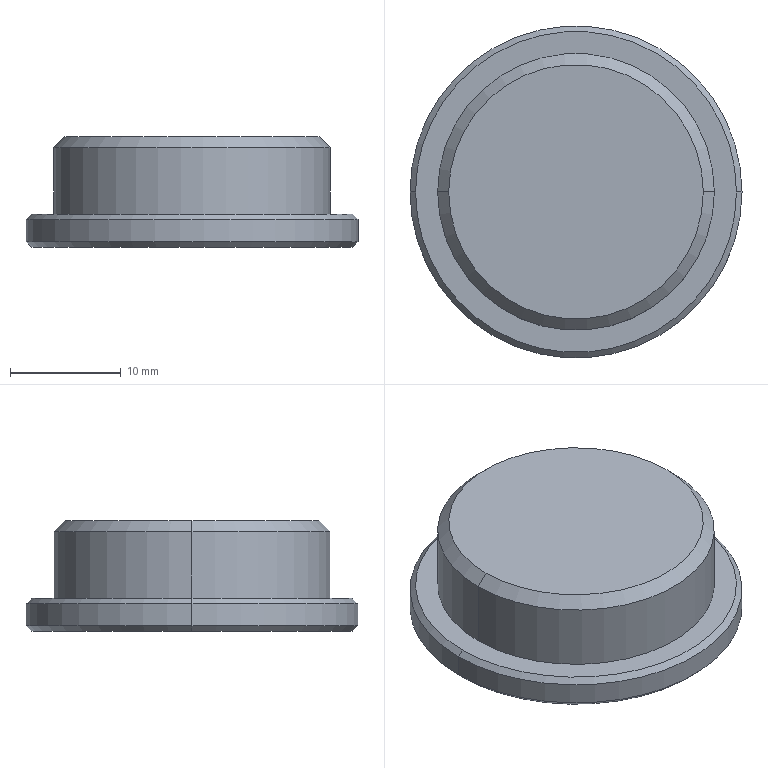Part | SolidWorks | features Chamfer 2, Revolution 1 | 1 solid | 13 faces | box 30 x 30 x 10 mm | volume 5495 mm3 | cone 6 | cylinder 4 | plane 3 | commonest cylinder face diameters 25 x2 30 x2
STEP:
#1=CARTESIAN_POINT('',(14.5,0.,-7.));
#2=VERTEX_POINT('',#1);
#3=CARTESIAN_POINT('',(-14.5,0.,-7.));
#4=VERTEX_POINT('',#3);
#5=CARTESIAN_POINT('',(0.,0.,-7.));
#6=DIRECTION('',(0.,0.,1.));
#7=DIRECTION('',(-1.,0.,0.));
#8=AXIS2_PLACEMENT_3D('',#5,#6,#7);
#9=CIRCLE('',#8,14.5);
#10=EDGE_CURVE('',#2,#4,#9,.T.);
#11=ORIENTED_EDGE('',*,*,#10,.F.);
#12=CARTESIAN_POINT('',(15.,0.,-7.5));
#13=VERTEX_POINT('',#12);
#14=CARTESIAN_POINT('',(14.5,0.,-7.));
#15=DIRECTION('',(0.7071,0.,-0.7071));
#16=VECTOR('',#15,1000.);
#17=LINE('',#14,#16);
#18=EDGE_CURVE('',#2,#13,#17,.T.);
#19=ORIENTED_EDGE('',*,*,#18,.T.);
#20=CARTESIAN_POINT('',(-15.,0.,-7.5));
#21=VERTEX_POINT('',#20);
#22=CARTESIAN_POINT('',(0.,0.,-7.5));
#23=DIRECTION('',(0.,0.,-1.));
#24=DIRECTION('',(-1.,0.,0.));
#25=AXIS2_PLACEMENT_3D('',#22,#23,#24);
#26=CIRCLE('',#25,15.);
#27=EDGE_CURVE('',#21,#13,#26,.T.);
#28=ORIENTED_EDGE('',*,*,#27,.F.);
#29=CARTESIAN_POINT('',(-14.5,0.,-7.));
#30=DIRECTION('',(-0.7071,0.,-0.7071));
#31=VECTOR('',#30,1000.);
#32=LINE('',#29,#31);
#33=EDGE_CURVE('',#4,#21,#32,.T.);
#34=ORIENTED_EDGE('',*,*,#33,.F.);
#35=EDGE_LOOP('',(#11,#19,#28,#34));
#36=FACE_OUTER_BOUND('',#35,.T.);
#37=CARTESIAN_POINT('',(0.,0.,-7.));
#38=DIRECTION('',(0.,0.,-1.));
#39=DIRECTION('',(-1.,0.,0.));
#40=AXIS2_PLACEMENT_3D('',#37,#38,#39);
#41=CONICAL_SURFACE('',#40,14.5,0.7854);
#42=ADVANCED_FACE('',(#36),#41,.T.);
#43=CARTESIAN_POINT('',(-14.5,0.,-10.));
#44=VERTEX_POINT('',#43);
#45=CARTESIAN_POINT('',(14.5,0.,-10.));
#46=VERTEX_POINT('',#45);
#47=CARTESIAN_POINT('',(0.,0.,-10.));
#48=DIRECTION('',(0.,0.,-1.));
#49=DIRECTION('',(1.,0.,0.));
#50=AXIS2_PLACEMENT_3D('',#47,#48,#49);
#51=CIRCLE('',#50,14.5);
#52=EDGE_CURVE('',#44,#46,#51,.T.);
#53=ORIENTED_EDGE('',*,*,#52,.F.);
#54=CARTESIAN_POINT('',(-15.,0.,-9.5));
#55=VERTEX_POINT('',#54);
#56=CARTESIAN_POINT('',(-15.,0.,-9.5));
#57=DIRECTION('',(-0.7071,0.,0.7071));
#58=VECTOR('',#57,1000.);
#59=LINE('',#56,#58);
#60=EDGE_CURVE('',#44,#55,#59,.T.);
#61=ORIENTED_EDGE('',*,*,#60,.T.);
#62=CARTESIAN_POINT('',(15.,0.,-9.5));
#63=VERTEX_POINT('',#62);
#64=CARTESIAN_POINT('',(0.,0.,-9.5));
#65=DIRECTION('',(0.,0.,1.));
#66=DIRECTION('',(1.,0.,0.));
#67=AXIS2_PLACEMENT_3D('',#64,#65,#66);
#68=CIRCLE('',#67,15.);
#69=EDGE_CURVE('',#63,#55,#68,.T.);
#70=ORIENTED_EDGE('',*,*,#69,.F.);
#71=CARTESIAN_POINT('',(15.,0.,-9.5));
#72=DIRECTION('',(0.7071,0.,0.7071));
#73=VECTOR('',#72,1000.);
#74=LINE('',#71,#73);
#75=EDGE_CURVE('',#46,#63,#74,.T.);
#76=ORIENTED_EDGE('',*,*,#75,.F.);
#77=EDGE_LOOP('',(#53,#61,#70,#76));
#78=FACE_OUTER_BOUND('',#77,.T.);
#79=CARTESIAN_POINT('',(0.,0.,-9.5));
#80=DIRECTION('',(0.,0.,1.));
#81=DIRECTION('',(1.,0.,0.));
#82=AXIS2_PLACEMENT_3D('',#79,#80,#81);
#83=CONICAL_SURFACE('',#82,15.,0.7854);
#84=ADVANCED_FACE('',(#78),#83,.T.);
#85=CARTESIAN_POINT('',(11.5,0.,0.));
#86=VERTEX_POINT('',#85);
#87=CARTESIAN_POINT('',(-11.5,0.,0.));
#88=VERTEX_POINT('',#87);
#89=CARTESIAN_POINT('',(0.,0.,0.));
#90=DIRECTION('',(0.,0.,1.));
#91=DIRECTION('',(-1.,0.,0.));
#92=AXIS2_PLACEMENT_3D('',#89,#90,#91);
#93=CIRCLE('',#92,11.5);
#94=EDGE_CURVE('',#86,#88,#93,.T.);
#95=ORIENTED_EDGE('',*,*,#94,.F.);
#96=CARTESIAN_POINT('',(12.5,0.,-1.));
#97=VERTEX_POINT('',#96);
#98=CARTESIAN_POINT('',(11.5,0.,0.));
#99=DIRECTION('',(0.7071,0.,-0.7071));
#100=VECTOR('',#99,1000.);
#101=LINE('',#98,#100);
#102=EDGE_CURVE('',#86,#97,#101,.T.);
#103=ORIENTED_EDGE('',*,*,#102,.T.);
#104=CARTESIAN_POINT('',(-12.5,0.,-1.));
#105=VERTEX_POINT('',#104);
#106=CARTESIAN_POINT('',(0.,0.,-1.));
#107=DIRECTION('',(0.,0.,-1.));
#108=DIRECTION('',(-1.,0.,0.));
#109=AXIS2_PLACEMENT_3D('',#106,#107,#108);
#110=CIRCLE('',#109,12.5);
#111=EDGE_CURVE('',#105,#97,#110,.T.);
#112=ORIENTED_EDGE('',*,*,#111,.F.);
#113=CARTESIAN_POINT('',(-11.5,0.,0.));
#114=DIRECTION('',(-0.7071,0.,-0.7071));
#115=VECTOR('',#114,1000.);
#116=LINE('',#113,#115);
#117=EDGE_CURVE('',#88,#105,#116,.T.);
#118=ORIENTED_EDGE('',*,*,#117,.F.);
#119=EDGE_LOOP('',(#95,#103,#112,#118));
#120=FACE_OUTER_BOUND('',#119,.T.);
#121=CARTESIAN_POINT('',(0.,0.,0.));
#122=DIRECTION('',(0.,0.,-1.));
#123=DIRECTION('',(-1.,0.,0.));
#124=AXIS2_PLACEMENT_3D('',#121,#122,#123);
#125=CONICAL_SURFACE('',#124,11.5,0.7854);
#126=ADVANCED_FACE('',(#120),#125,.T.);
#127=CARTESIAN_POINT('',(12.5,0.,-7.));
#128=VERTEX_POINT('',#127);
#129=CARTESIAN_POINT('',(-12.5,0.,-7.));
#130=VERTEX_POINT('',#129);
#131=CARTESIAN_POINT('',(0.,0.,-7.));
#132=DIRECTION('',(0.,0.,1.));
#133=DIRECTION('',(1.,0.,0.));
#134=AXIS2_PLACEMENT_3D('',#131,#132,#133);
#135=CIRCLE('',#134,12.5);
#136=EDGE_CURVE('',#128,#130,#135,.T.);
#137=ORIENTED_EDGE('',*,*,#136,.T.);
#138=CARTESIAN_POINT('',(-12.5,0.,0.));
#139=DIRECTION('',(0.,0.,1.));
#140=VECTOR('',#139,1000.);
#141=LINE('',#138,#140);
#142=EDGE_CURVE('',#130,#105,#141,.T.);
#143=ORIENTED_EDGE('',*,*,#142,.T.);
#144=ORIENTED_EDGE('',*,*,#111,.T.);
#145=CARTESIAN_POINT('',(12.5,0.,0.));
#146=DIRECTION('',(0.,0.,1.));
#147=VECTOR('',#146,1000.);
#148=LINE('',#145,#147);
#149=EDGE_CURVE('',#128,#97,#148,.T.);
#150=ORIENTED_EDGE('',*,*,#149,.F.);
#151=EDGE_LOOP('',(#137,#143,#144,#150));
#152=FACE_OUTER_BOUND('',#151,.T.);
#153=CARTESIAN_POINT('',(0.,0.,0.));
#154=DIRECTION('',(0.,0.,1.));
#155=DIRECTION('',(1.,0.,0.));
#156=AXIS2_PLACEMENT_3D('',#153,#154,#155);
#157=CYLINDRICAL_SURFACE('',#156,12.5);
#158=ADVANCED_FACE('',(#152),#157,.T.);
#159=ORIENTED_EDGE('',*,*,#69,.T.);
#160=CARTESIAN_POINT('',(-15.,0.,0.));
#161=DIRECTION('',(0.,0.,1.));
#162=VECTOR('',#161,1000.);
#163=LINE('',#160,#162);
#164=EDGE_CURVE('',#55,#21,#163,.T.);
#165=ORIENTED_EDGE('',*,*,#164,.T.);
#166=ORIENTED_EDGE('',*,*,#27,.T.);
#167=CARTESIAN_POINT('',(15.,0.,0.));
#168=DIRECTION('',(0.,0.,1.));
#169=VECTOR('',#168,1000.);
#170=LINE('',#167,#169);
#171=EDGE_CURVE('',#63,#13,#170,.T.);
#172=ORIENTED_EDGE('',*,*,#171,.F.);
#173=EDGE_LOOP('',(#159,#165,#166,#172));
#174=FACE_OUTER_BOUND('',#173,.T.);
#175=CARTESIAN_POINT('',(0.,0.,0.));
#176=DIRECTION('',(0.,0.,1.));
#177=DIRECTION('',(1.,0.,0.));
#178=AXIS2_PLACEMENT_3D('',#175,#176,#177);
#179=CYLINDRICAL_SURFACE('',#178,15.);
#180=ADVANCED_FACE('',(#174),#179,.T.);
#181=CARTESIAN_POINT('',(0.,0.,-10.));
#182=DIRECTION('',(0.,0.,-1.));
#183=DIRECTION('',(1.,0.,0.));
#184=AXIS2_PLACEMENT_3D('',#181,#182,#183);
#185=CIRCLE('',#184,14.5);
#186=EDGE_CURVE('',#46,#44,#185,.T.);
#187=ORIENTED_EDGE('',*,*,#186,.T.);
#188=ORIENTED_EDGE('',*,*,#52,.T.);
#189=EDGE_LOOP('',(#187,#188));
#190=FACE_OUTER_BOUND('',#189,.T.);
#191=CARTESIAN_POINT('',(0.,0.,-10.));
#192=DIRECTION('',(0.,0.,1.));
#193=DIRECTION('',(1.,0.,0.));
#194=AXIS2_PLACEMENT_3D('',#191,#192,#193);
#195=PLANE('',#194);
#196=ADVANCED_FACE('',(#190),#195,.F.);
#197=ORIENTED_EDGE('',*,*,#164,.F.);
#198=CARTESIAN_POINT('',(0.,0.,-9.5));
#199=DIRECTION('',(0.,0.,1.));
#200=DIRECTION('',(1.,0.,0.));
#201=AXIS2_PLACEMENT_3D('',#198,#199,#200);
#202=CIRCLE('',#201,15.);
#203=EDGE_CURVE('',#55,#63,#202,.T.);
#204=ORIENTED_EDGE('',*,*,#203,.T.);
#205=ORIENTED_EDGE('',*,*,#171,.T.);
#206=CARTESIAN_POINT('',(0.,0.,-7.5));
#207=DIRECTION('',(0.,0.,-1.));
#208=DIRECTION('',(-1.,0.,0.));
#209=AXIS2_PLACEMENT_3D('',#206,#207,#208);
#210=CIRCLE('',#209,15.);
#211=EDGE_CURVE('',#13,#21,#210,.T.);
#212=ORIENTED_EDGE('',*,*,#211,.T.);
#213=EDGE_LOOP('',(#197,#204,#205,#212));
#214=FACE_OUTER_BOUND('',#213,.T.);
#215=CARTESIAN_POINT('',(0.,0.,0.));
#216=DIRECTION('',(0.,0.,1.));
#217=DIRECTION('',(1.,0.,0.));
#218=AXIS2_PLACEMENT_3D('',#215,#216,#217);
#219=CYLINDRICAL_SURFACE('',#218,15.);
#220=ADVANCED_FACE('',(#214),#219,.T.);
#221=CARTESIAN_POINT('',(0.,0.,-7.));
#222=DIRECTION('',(0.,0.,1.));
#223=DIRECTION('',(-1.,0.,0.));
#224=AXIS2_PLACEMENT_3D('',#221,#222,#223);
#225=CIRCLE('',#224,14.5);
#226=EDGE_CURVE('',#4,#2,#225,.T.);
#227=ORIENTED_EDGE('',*,*,#226,.T.);
#228=ORIENTED_EDGE('',*,*,#10,.T.);
#229=EDGE_LOOP('',(#227,#228));
#230=FACE_OUTER_BOUND('',#229,.T.);
#231=ORIENTED_EDGE('',*,*,#136,.F.);
#232=CARTESIAN_POINT('',(0.,0.,-7.));
#233=DIRECTION('',(0.,0.,1.));
#234=DIRECTION('',(1.,0.,0.));
#235=AXIS2_PLACEMENT_3D('',#232,#233,#234);
#236=CIRCLE('',#235,12.5);
#237=EDGE_CURVE('',#130,#128,#236,.T.);
#238=ORIENTED_EDGE('',*,*,#237,.F.);
#239=EDGE_LOOP('',(#231,#238));
#240=FACE_BOUND('',#239,.T.);
#241=CARTESIAN_POINT('',(0.,15.,-7.));
#242=DIRECTION('',(0.,0.,-1.));
#243=DIRECTION('',(-1.,0.,0.));
#244=AXIS2_PLACEMENT_3D('',#241,#242,#243);
#245=PLANE('',#244);
#246=ADVANCED_FACE('',(#230,#240),#245,.F.);
#247=ORIENTED_EDGE('',*,*,#142,.F.);
#248=ORIENTED_EDGE('',*,*,#237,.T.);
#249=ORIENTED_EDGE('',*,*,#149,.T.);
#250=CARTESIAN_POINT('',(0.,0.,-1.));
#251=DIRECTION('',(0.,0.,-1.));
#252=DIRECTION('',(-1.,0.,0.));
#253=AXIS2_PLACEMENT_3D('',#250,#251,#252);
#254=CIRCLE('',#253,12.5);
#255=EDGE_CURVE('',#97,#105,#254,.T.);
#256=ORIENTED_EDGE('',*,*,#255,.T.);
#257=EDGE_LOOP('',(#247,#248,#249,#256));
#258=FACE_OUTER_BOUND('',#257,.T.);
#259=CARTESIAN_POINT('',(0.,0.,0.));
#260=DIRECTION('',(0.,0.,1.));
#261=DIRECTION('',(1.,0.,0.));
#262=AXIS2_PLACEMENT_3D('',#259,#260,#261);
#263=CYLINDRICAL_SURFACE('',#262,12.5);
#264=ADVANCED_FACE('',(#258),#263,.T.);
#265=CARTESIAN_POINT('',(0.,0.,0.));
#266=DIRECTION('',(0.,0.,1.));
#267=DIRECTION('',(-1.,0.,0.));
#268=AXIS2_PLACEMENT_3D('',#265,#266,#267);
#269=CIRCLE('',#268,11.5);
#270=EDGE_CURVE('',#88,#86,#269,.T.);
#271=ORIENTED_EDGE('',*,*,#270,.T.);
#272=ORIENTED_EDGE('',*,*,#94,.T.);
#273=EDGE_LOOP('',(#271,#272));
#274=FACE_OUTER_BOUND('',#273,.T.);
#275=CARTESIAN_POINT('',(0.,12.5,0.));
#276=DIRECTION('',(0.,0.,-1.));
#277=DIRECTION('',(-1.,0.,0.));
#278=AXIS2_PLACEMENT_3D('',#275,#276,#277);
#279=PLANE('',#278);
#280=ADVANCED_FACE('',(#274),#279,.F.);
#281=ORIENTED_EDGE('',*,*,#102,.F.);
#282=ORIENTED_EDGE('',*,*,#270,.F.);
#283=ORIENTED_EDGE('',*,*,#117,.T.);
#284=ORIENTED_EDGE('',*,*,#255,.F.);
#285=EDGE_LOOP('',(#281,#282,#283,#284));
#286=FACE_OUTER_BOUND('',#285,.T.);
#287=CARTESIAN_POINT('',(0.,0.,0.));
#288=DIRECTION('',(0.,0.,-1.));
#289=DIRECTION('',(-1.,0.,0.));
#290=AXIS2_PLACEMENT_3D('',#287,#288,#289);
#291=CONICAL_SURFACE('',#290,11.5,0.7854);
#292=ADVANCED_FACE('',(#286),#291,.T.);
#293=ORIENTED_EDGE('',*,*,#60,.F.);
#294=ORIENTED_EDGE('',*,*,#186,.F.);
#295=ORIENTED_EDGE('',*,*,#75,.T.);
#296=ORIENTED_EDGE('',*,*,#203,.F.);
#297=EDGE_LOOP('',(#293,#294,#295,#296));
#298=FACE_OUTER_BOUND('',#297,.T.);
#299=CARTESIAN_POINT('',(0.,0.,-9.5));
#300=DIRECTION('',(0.,0.,1.));
#301=DIRECTION('',(1.,0.,0.));
#302=AXIS2_PLACEMENT_3D('',#299,#300,#301);
#303=CONICAL_SURFACE('',#302,15.,0.7854);
#304=ADVANCED_FACE('',(#298),#303,.T.);
#305=ORIENTED_EDGE('',*,*,#18,.F.);
#306=ORIENTED_EDGE('',*,*,#226,.F.);
#307=ORIENTED_EDGE('',*,*,#33,.T.);
#308=ORIENTED_EDGE('',*,*,#211,.F.);
#309=EDGE_LOOP('',(#305,#306,#307,#308));
#310=FACE_OUTER_BOUND('',#309,.T.);
#311=CARTESIAN_POINT('',(0.,0.,-7.));
#312=DIRECTION('',(0.,0.,-1.));
#313=DIRECTION('',(-1.,0.,0.));
#314=AXIS2_PLACEMENT_3D('',#311,#312,#313);
#315=CONICAL_SURFACE('',#314,14.5,0.7854);
#316=ADVANCED_FACE('',(#310),#315,.T.);
#317=CLOSED_SHELL('',(#42,#84,#126,#158,#180,#196,#220,#246,#264,#280,#292,#304,#316));
#318=MANIFOLD_SOLID_BREP('',#317);
#319=CARTESIAN_POINT('',(0.,0.,0.));
#320=DIRECTION('',(0.,0.,1.));
#321=DIRECTION('',(1.,0.,0.));
#322=AXIS2_PLACEMENT_3D('',#319,#320,#321);
#323=(LENGTH_UNIT()NAMED_UNIT(*)SI_UNIT(.MILLI.,.METRE.));
#324=UNCERTAINTY_MEASURE_WITH_UNIT(LENGTH_MEASURE(0.00001),#323,'','');
#325=(NAMED_UNIT(*)PLANE_ANGLE_UNIT()SI_UNIT($,.RADIAN.));
#326=(NAMED_UNIT(*)SI_UNIT($,.STERADIAN.)SOLID_ANGLE_UNIT());
#327=(GEOMETRIC_REPRESENTATION_CONTEXT(3)GLOBAL_UNCERTAINTY_ASSIGNED_CONTEXT((#324))GLOBAL_UNIT_ASSIGNED_CONTEXT((#323,#325,#326))REPRESENTATION_CONTEXT('',''));
#328=ADVANCED_BREP_SHAPE_REPRESENTATION('',(#318,#322),#327);